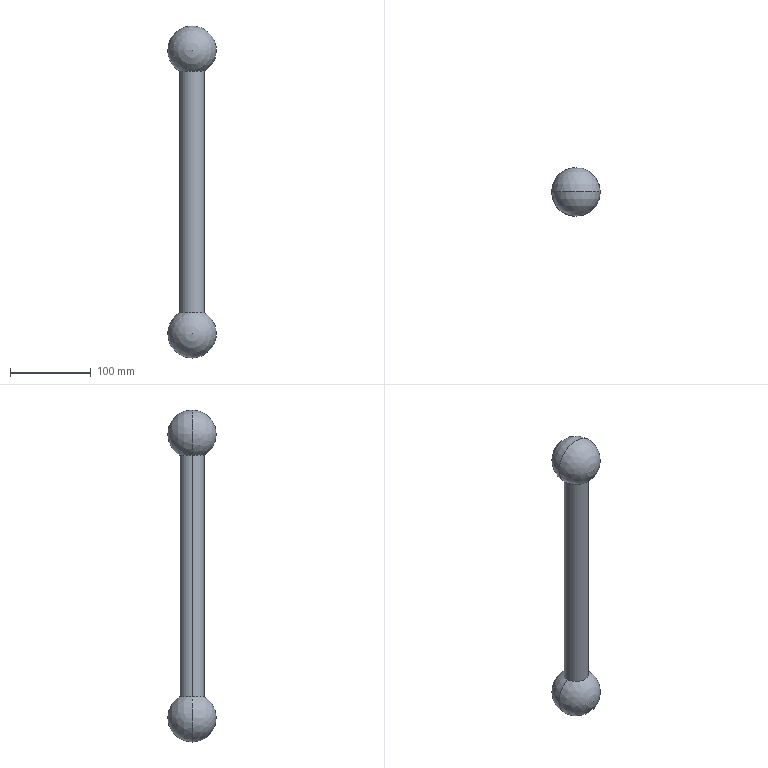Part | SolidWorks | features Extrusion 1, MirrorPattern 1, Revolution 1 | 1 solid | 6 faces | box 60 x 60 x 410 mm | volume 433957 mm3 | sphere 4 | cylinder 2 | commonest cylinder face diameters 30 x2
STEP:
#1=CARTESIAN_POINT('',(-15.,0.,149.019));
#2=VERTEX_POINT('',#1);
#3=CARTESIAN_POINT('',(15.,0.,149.019));
#4=VERTEX_POINT('',#3);
#5=CARTESIAN_POINT('',(0.,0.,149.019));
#6=DIRECTION('',(0.,0.,1.));
#7=DIRECTION('',(1.,0.,0.));
#8=AXIS2_PLACEMENT_3D('',#5,#6,#7);
#9=CIRCLE('',#8,15.);
#10=EDGE_CURVE('',#2,#4,#9,.T.);
#11=ORIENTED_EDGE('',*,*,#10,.T.);
#12=CARTESIAN_POINT('',(0.,0.,205.));
#13=VERTEX_POINT('',#12);
#14=CARTESIAN_POINT('',(0.,0.,175.));
#15=DIRECTION('',(0.,-1.,0.));
#16=DIRECTION('',(1.,0.,0.));
#17=AXIS2_PLACEMENT_3D('',#14,#15,#16);
#18=CIRCLE('',#17,30.);
#19=EDGE_CURVE('',#4,#13,#18,.T.);
#20=ORIENTED_EDGE('',*,*,#19,.T.);
#21=CARTESIAN_POINT('',(0.,0.,175.));
#22=DIRECTION('',(0.,1.,0.));
#23=DIRECTION('',(0.,0.,1.));
#24=AXIS2_PLACEMENT_3D('',#21,#22,#23);
#25=CIRCLE('',#24,30.);
#26=EDGE_CURVE('',#2,#13,#25,.T.);
#27=ORIENTED_EDGE('',*,*,#26,.F.);
#28=EDGE_LOOP('',(#11,#20,#27));
#29=FACE_OUTER_BOUND('',#28,.T.);
#30=CARTESIAN_POINT('',(0.,0.,175.));
#31=DIRECTION('',(0.,-1.,0.));
#32=DIRECTION('',(-1.,0.,0.));
#33=AXIS2_PLACEMENT_3D('',#30,#31,#32);
#34=SPHERICAL_SURFACE('',#33,30.);
#35=ADVANCED_FACE('',(#29),#34,.T.);
#36=CARTESIAN_POINT('',(-15.,0.,-149.019));
#37=VERTEX_POINT('',#36);
#38=CARTESIAN_POINT('',(15.,0.,-149.019));
#39=VERTEX_POINT('',#38);
#40=CARTESIAN_POINT('',(0.,0.,-149.019));
#41=DIRECTION('',(0.,0.,-1.));
#42=DIRECTION('',(-1.,0.,0.));
#43=AXIS2_PLACEMENT_3D('',#40,#41,#42);
#44=CIRCLE('',#43,15.);
#45=EDGE_CURVE('',#37,#39,#44,.T.);
#46=ORIENTED_EDGE('',*,*,#45,.T.);
#47=CARTESIAN_POINT('',(0.,0.,-205.));
#48=VERTEX_POINT('',#47);
#49=CARTESIAN_POINT('',(0.,0.,-175.));
#50=DIRECTION('',(0.,1.,0.));
#51=DIRECTION('',(-1.,0.,0.));
#52=AXIS2_PLACEMENT_3D('',#49,#50,#51);
#53=CIRCLE('',#52,30.);
#54=EDGE_CURVE('',#39,#48,#53,.T.);
#55=ORIENTED_EDGE('',*,*,#54,.T.);
#56=CARTESIAN_POINT('',(0.,0.,-175.));
#57=DIRECTION('',(0.,-1.,0.));
#58=DIRECTION('',(0.,0.,-1.));
#59=AXIS2_PLACEMENT_3D('',#56,#57,#58);
#60=CIRCLE('',#59,30.);
#61=EDGE_CURVE('',#37,#48,#60,.T.);
#62=ORIENTED_EDGE('',*,*,#61,.F.);
#63=EDGE_LOOP('',(#46,#55,#62));
#64=FACE_OUTER_BOUND('',#63,.T.);
#65=CARTESIAN_POINT('',(0.,0.,-175.));
#66=DIRECTION('',(0.,1.,0.));
#67=DIRECTION('',(-1.,0.,0.));
#68=AXIS2_PLACEMENT_3D('',#65,#66,#67);
#69=SPHERICAL_SURFACE('',#68,30.);
#70=ADVANCED_FACE('',(#64),#69,.T.);
#71=CARTESIAN_POINT('',(0.,0.,149.019));
#72=DIRECTION('',(0.,0.,1.));
#73=DIRECTION('',(1.,0.,0.));
#74=AXIS2_PLACEMENT_3D('',#71,#72,#73);
#75=CIRCLE('',#74,15.);
#76=EDGE_CURVE('',#4,#2,#75,.T.);
#77=ORIENTED_EDGE('',*,*,#76,.F.);
#78=CARTESIAN_POINT('',(15.,0.,150.));
#79=DIRECTION('',(0.,0.,-1.));
#80=VECTOR('',#79,1000.);
#81=LINE('',#78,#80);
#82=EDGE_CURVE('',#4,#39,#81,.T.);
#83=ORIENTED_EDGE('',*,*,#82,.T.);
#84=ORIENTED_EDGE('',*,*,#45,.F.);
#85=CARTESIAN_POINT('',(-15.,0.,150.));
#86=DIRECTION('',(0.,0.,-1.));
#87=VECTOR('',#86,1000.);
#88=LINE('',#85,#87);
#89=EDGE_CURVE('',#2,#37,#88,.T.);
#90=ORIENTED_EDGE('',*,*,#89,.F.);
#91=EDGE_LOOP('',(#77,#83,#84,#90));
#92=FACE_OUTER_BOUND('',#91,.T.);
#93=CARTESIAN_POINT('',(0.,0.,150.));
#94=DIRECTION('',(0.,0.,-1.));
#95=DIRECTION('',(-1.,0.,0.));
#96=AXIS2_PLACEMENT_3D('',#93,#94,#95);
#97=CYLINDRICAL_SURFACE('',#96,15.);
#98=ADVANCED_FACE('',(#92),#97,.T.);
#99=ORIENTED_EDGE('',*,*,#82,.F.);
#100=ORIENTED_EDGE('',*,*,#10,.F.);
#101=ORIENTED_EDGE('',*,*,#89,.T.);
#102=CARTESIAN_POINT('',(0.,0.,-149.019));
#103=DIRECTION('',(0.,0.,-1.));
#104=DIRECTION('',(-1.,0.,0.));
#105=AXIS2_PLACEMENT_3D('',#102,#103,#104);
#106=CIRCLE('',#105,15.);
#107=EDGE_CURVE('',#39,#37,#106,.T.);
#108=ORIENTED_EDGE('',*,*,#107,.F.);
#109=EDGE_LOOP('',(#99,#100,#101,#108));
#110=FACE_OUTER_BOUND('',#109,.T.);
#111=CARTESIAN_POINT('',(0.,0.,150.));
#112=DIRECTION('',(0.,0.,-1.));
#113=DIRECTION('',(-1.,0.,0.));
#114=AXIS2_PLACEMENT_3D('',#111,#112,#113);
#115=CYLINDRICAL_SURFACE('',#114,15.);
#116=ADVANCED_FACE('',(#110),#115,.T.);
#117=ORIENTED_EDGE('',*,*,#54,.F.);
#118=ORIENTED_EDGE('',*,*,#107,.T.);
#119=ORIENTED_EDGE('',*,*,#61,.T.);
#120=EDGE_LOOP('',(#117,#118,#119));
#121=FACE_OUTER_BOUND('',#120,.T.);
#122=CARTESIAN_POINT('',(0.,0.,-175.));
#123=DIRECTION('',(0.,1.,0.));
#124=DIRECTION('',(-1.,0.,0.));
#125=AXIS2_PLACEMENT_3D('',#122,#123,#124);
#126=SPHERICAL_SURFACE('',#125,30.);
#127=ADVANCED_FACE('',(#121),#126,.T.);
#128=ORIENTED_EDGE('',*,*,#19,.F.);
#129=ORIENTED_EDGE('',*,*,#76,.T.);
#130=ORIENTED_EDGE('',*,*,#26,.T.);
#131=EDGE_LOOP('',(#128,#129,#130));
#132=FACE_OUTER_BOUND('',#131,.T.);
#133=CARTESIAN_POINT('',(0.,0.,175.));
#134=DIRECTION('',(0.,-1.,0.));
#135=DIRECTION('',(-1.,0.,0.));
#136=AXIS2_PLACEMENT_3D('',#133,#134,#135);
#137=SPHERICAL_SURFACE('',#136,30.);
#138=ADVANCED_FACE('',(#132),#137,.T.);
#139=CLOSED_SHELL('',(#35,#70,#98,#116,#127,#138));
#140=MANIFOLD_SOLID_BREP('',#139);
#141=CARTESIAN_POINT('',(0.,0.,0.));
#142=DIRECTION('',(0.,0.,1.));
#143=DIRECTION('',(1.,0.,0.));
#144=AXIS2_PLACEMENT_3D('',#141,#142,#143);
#145=(LENGTH_UNIT()NAMED_UNIT(*)SI_UNIT(.MILLI.,.METRE.));
#146=UNCERTAINTY_MEASURE_WITH_UNIT(LENGTH_MEASURE(0.00001),#145,'','');
#147=(NAMED_UNIT(*)PLANE_ANGLE_UNIT()SI_UNIT($,.RADIAN.));
#148=(NAMED_UNIT(*)SI_UNIT($,.STERADIAN.)SOLID_ANGLE_UNIT());
#149=(GEOMETRIC_REPRESENTATION_CONTEXT(3)GLOBAL_UNCERTAINTY_ASSIGNED_CONTEXT((#146))GLOBAL_UNIT_ASSIGNED_CONTEXT((#145,#147,#148))REPRESENTATION_CONTEXT('',''));
#150=ADVANCED_BREP_SHAPE_REPRESENTATION('',(#140,#144),#149);